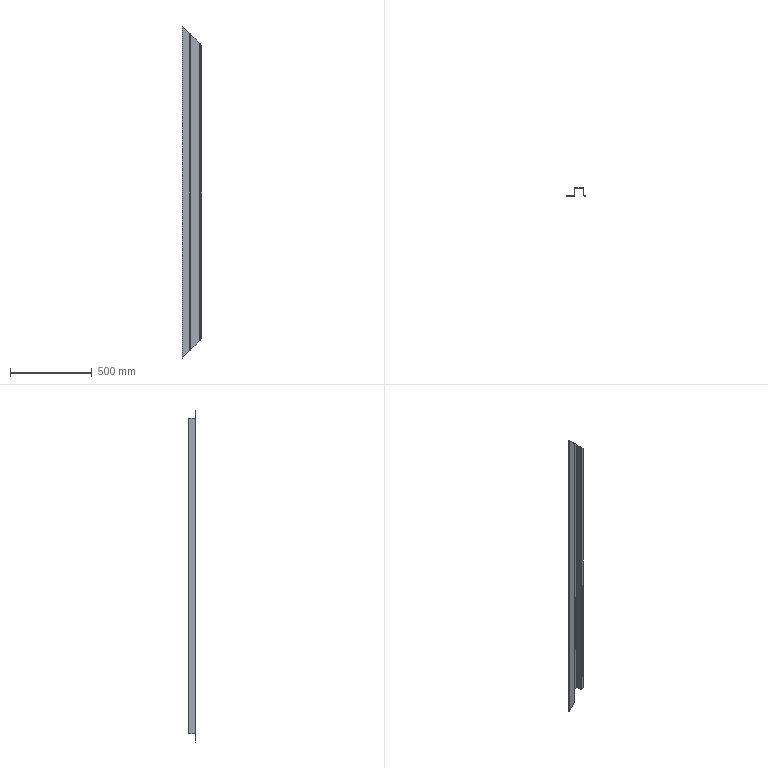Part | STEP file | 750038412 | 1 solid | 38 faces | box 120 x 46.5 x 2028 mm | volume 584981 mm3 | plane 22 | cylinder 8 | spline 8 | commonest cylinder face diameters 3 x4 6 x4
STEP:
#1=CARTESIAN_POINT('',(-14.5,45.,-908.5));
#2=VERTEX_POINT('',#1);
#3=CARTESIAN_POINT('',(-14.5,45.,908.5));
#4=VERTEX_POINT('',#3);
#5=CARTESIAN_POINT('',(-14.5,45.,1014.));
#6=DIRECTION('',(0.,0.,1.));
#7=VECTOR('',#6,1000.);
#8=LINE('',#5,#7);
#9=EDGE_CURVE('',#2,#4,#8,.T.);
#10=ORIENTED_EDGE('',*,*,#9,.F.);
#11=CARTESIAN_POINT('',(-68.5,45.,-962.5));
#12=VERTEX_POINT('',#11);
#13=CARTESIAN_POINT('',(-68.5,45.,-962.5));
#14=DIRECTION('',(0.7071,0.,0.7071));
#15=VECTOR('',#14,1000.);
#16=LINE('',#13,#15);
#17=EDGE_CURVE('',#12,#2,#16,.T.);
#18=ORIENTED_EDGE('',*,*,#17,.F.);
#19=CARTESIAN_POINT('',(-68.5,45.,962.5));
#20=VERTEX_POINT('',#19);
#21=CARTESIAN_POINT('',(-68.5,45.,1014.));
#22=DIRECTION('',(0.,0.,-1.));
#23=VECTOR('',#22,1000.);
#24=LINE('',#21,#23);
#25=EDGE_CURVE('',#20,#12,#24,.T.);
#26=ORIENTED_EDGE('',*,*,#25,.F.);
#27=CARTESIAN_POINT('',(-14.5,45.,908.5));
#28=DIRECTION('',(-0.7071,0.,0.7071));
#29=VECTOR('',#28,1000.);
#30=LINE('',#27,#29);
#31=EDGE_CURVE('',#4,#20,#30,.T.);
#32=ORIENTED_EDGE('',*,*,#31,.F.);
#33=EDGE_LOOP('',(#10,#18,#26,#32));
#34=FACE_OUTER_BOUND('',#33,.T.);
#35=CARTESIAN_POINT('',(-11.5,45.,1014.));
#36=DIRECTION('',(0.,-1.,0.));
#37=DIRECTION('',(1.,0.,0.));
#38=AXIS2_PLACEMENT_3D('',#35,#36,#37);
#39=PLANE('',#38);
#40=ADVANCED_FACE('',(#34),#39,.F.);
#41=CARTESIAN_POINT('',(-68.5,43.5,962.5));
#42=VERTEX_POINT('',#41);
#43=CARTESIAN_POINT('',(-68.5,44.25,962.5));
#44=DIRECTION('',(0.,-1.,0.));
#45=VECTOR('',#44,1000.);
#46=LINE('',#43,#45);
#47=EDGE_CURVE('',#20,#42,#46,.T.);
#48=ORIENTED_EDGE('',*,*,#47,.T.);
#49=CARTESIAN_POINT('',(-14.5,43.5,908.5));
#50=VERTEX_POINT('',#49);
#51=CARTESIAN_POINT('',(-65.75,43.5,959.75));
#52=DIRECTION('',(0.7071,0.,-0.7071));
#53=VECTOR('',#52,1000.);
#54=LINE('',#51,#53);
#55=EDGE_CURVE('',#42,#50,#54,.T.);
#56=ORIENTED_EDGE('',*,*,#55,.T.);
#57=CARTESIAN_POINT('',(-14.5,44.25,908.5));
#58=DIRECTION('',(0.,1.,0.));
#59=VECTOR('',#58,1000.);
#60=LINE('',#57,#59);
#61=EDGE_CURVE('',#50,#4,#60,.T.);
#62=ORIENTED_EDGE('',*,*,#61,.T.);
#63=ORIENTED_EDGE('',*,*,#31,.T.);
#64=EDGE_LOOP('',(#48,#56,#62,#63));
#65=FACE_OUTER_BOUND('',#64,.T.);
#66=CARTESIAN_POINT('',(-65.75,45.,959.75));
#67=DIRECTION('',(0.7071,0.,0.7071));
#68=DIRECTION('',(0.7071,0.,-0.7071));
#69=AXIS2_PLACEMENT_3D('',#66,#67,#68);
#70=PLANE('',#69);
#71=ADVANCED_FACE('',(#65),#70,.T.);
#72=CARTESIAN_POINT('',(-11.5,42.,-905.5));
#73=VERTEX_POINT('',#72);
#74=CARTESIAN_POINT('',(-11.5,42.,-905.5));
#75=CARTESIAN_POINT('',(-11.5,43.5,-905.5));
#76=CARTESIAN_POINT('',(-12.5,45.,-906.5));
#77=CARTESIAN_POINT('',(-14.5,45.,-908.5));
#78=(BOUNDED_CURVE()B_SPLINE_CURVE(3,(#74,#75,#76,#77),.UNSPECIFIED.,.F.,.T.)B_SPLINE_CURVE_WITH_KNOTS((4,4),(0.,0.005726),.UNSPECIFIED.)CURVE()GEOMETRIC_REPRESENTATION_ITEM()RATIONAL_B_SPLINE_CURVE((1.,0.6667,0.5,0.5))REPRESENTATION_ITEM(''));
#79=EDGE_CURVE('',#73,#2,#78,.T.);
#80=ORIENTED_EDGE('',*,*,#79,.T.);
#81=ORIENTED_EDGE('',*,*,#9,.T.);
#82=CARTESIAN_POINT('',(-11.5,42.,905.5));
#83=VERTEX_POINT('',#82);
#84=CARTESIAN_POINT('',(-14.5,45.,908.5));
#85=CARTESIAN_POINT('',(-12.5,45.,906.5));
#86=CARTESIAN_POINT('',(-11.5,43.5,905.5));
#87=CARTESIAN_POINT('',(-11.5,42.,905.5));
#88=(BOUNDED_CURVE()B_SPLINE_CURVE(3,(#84,#85,#86,#87),.UNSPECIFIED.,.F.,.T.)B_SPLINE_CURVE_WITH_KNOTS((4,4),(0.,0.005675),.UNSPECIFIED.)CURVE()GEOMETRIC_REPRESENTATION_ITEM()RATIONAL_B_SPLINE_CURVE((0.5,0.5,0.6667,1.))REPRESENTATION_ITEM(''));
#89=EDGE_CURVE('',#4,#83,#88,.T.);
#90=ORIENTED_EDGE('',*,*,#89,.T.);
#91=CARTESIAN_POINT('',(-11.5,42.,1014.));
#92=DIRECTION('',(0.,0.,-1.));
#93=VECTOR('',#92,1000.);
#94=LINE('',#91,#93);
#95=EDGE_CURVE('',#83,#73,#94,.T.);
#96=ORIENTED_EDGE('',*,*,#95,.T.);
#97=EDGE_LOOP('',(#80,#81,#90,#96));
#98=FACE_OUTER_BOUND('',#97,.T.);
#99=CARTESIAN_POINT('',(-14.5,42.,1014.));
#100=DIRECTION('',(0.,0.,-1.));
#101=DIRECTION('',(-1.,0.,0.));
#102=AXIS2_PLACEMENT_3D('',#99,#100,#101);
#103=CYLINDRICAL_SURFACE('',#102,3.);
#104=ADVANCED_FACE('',(#98),#103,.T.);
#105=CARTESIAN_POINT('',(-14.5,43.5,-908.5));
#106=VERTEX_POINT('',#105);
#107=CARTESIAN_POINT('',(-14.5,45.,-908.5));
#108=DIRECTION('',(0.,-1.,0.));
#109=VECTOR('',#108,1000.);
#110=LINE('',#107,#109);
#111=EDGE_CURVE('',#2,#106,#110,.T.);
#112=ORIENTED_EDGE('',*,*,#111,.T.);
#113=CARTESIAN_POINT('',(-68.5,43.5,-962.5));
#114=VERTEX_POINT('',#113);
#115=CARTESIAN_POINT('',(948.25,43.5,54.25));
#116=DIRECTION('',(-0.7071,0.,-0.7071));
#117=VECTOR('',#116,1000.);
#118=LINE('',#115,#117);
#119=EDGE_CURVE('',#106,#114,#118,.T.);
#120=ORIENTED_EDGE('',*,*,#119,.T.);
#121=CARTESIAN_POINT('',(-68.5,44.25,-962.5));
#122=DIRECTION('',(0.,1.,0.));
#123=VECTOR('',#122,1000.);
#124=LINE('',#121,#123);
#125=EDGE_CURVE('',#114,#12,#124,.T.);
#126=ORIENTED_EDGE('',*,*,#125,.T.);
#127=ORIENTED_EDGE('',*,*,#17,.T.);
#128=EDGE_LOOP('',(#112,#120,#126,#127));
#129=FACE_OUTER_BOUND('',#128,.T.);
#130=CARTESIAN_POINT('',(948.25,45.,54.25));
#131=DIRECTION('',(0.7071,0.,-0.7071));
#132=DIRECTION('',(-0.7071,0.,-0.7071));
#133=AXIS2_PLACEMENT_3D('',#130,#131,#132);
#134=PLANE('',#133);
#135=ADVANCED_FACE('',(#129),#134,.T.);
#136=CARTESIAN_POINT('',(-71.5,42.,-964.));
#137=VERTEX_POINT('',#136);
#138=CARTESIAN_POINT('',(-68.5,45.,-962.5));
#139=CARTESIAN_POINT('',(-70.5,45.,-963.5));
#140=CARTESIAN_POINT('',(-71.5,43.5,-964.));
#141=CARTESIAN_POINT('',(-71.5,42.,-964.));
#142=(BOUNDED_CURVE()B_SPLINE_CURVE(3,(#138,#139,#140,#141),.UNSPECIFIED.,.F.,.T.)B_SPLINE_CURVE_WITH_KNOTS((4,4),(0.,0.004967),.UNSPECIFIED.)CURVE()GEOMETRIC_REPRESENTATION_ITEM()RATIONAL_B_SPLINE_CURVE((0.5,0.5,0.6667,1.))REPRESENTATION_ITEM(''));
#143=EDGE_CURVE('',#12,#137,#142,.T.);
#144=ORIENTED_EDGE('',*,*,#143,.T.);
#145=CARTESIAN_POINT('',(-71.5,42.,964.));
#146=VERTEX_POINT('',#145);
#147=CARTESIAN_POINT('',(-71.5,42.,1014.));
#148=DIRECTION('',(0.,0.,1.));
#149=VECTOR('',#148,1000.);
#150=LINE('',#147,#149);
#151=EDGE_CURVE('',#137,#146,#150,.T.);
#152=ORIENTED_EDGE('',*,*,#151,.T.);
#153=CARTESIAN_POINT('',(-71.5,42.,964.));
#154=CARTESIAN_POINT('',(-71.5,43.5,964.));
#155=CARTESIAN_POINT('',(-70.5,45.,963.5));
#156=CARTESIAN_POINT('',(-68.5,45.,962.5));
#157=(BOUNDED_CURVE()B_SPLINE_CURVE(3,(#153,#154,#155,#156),.UNSPECIFIED.,.F.,.F.)B_SPLINE_CURVE_WITH_KNOTS((4,4),(0.,0.00499),.UNSPECIFIED.)CURVE()GEOMETRIC_REPRESENTATION_ITEM()RATIONAL_B_SPLINE_CURVE((1.,0.6667,0.5,0.5))REPRESENTATION_ITEM(''));
#158=EDGE_CURVE('',#146,#20,#157,.T.);
#159=ORIENTED_EDGE('',*,*,#158,.T.);
#160=ORIENTED_EDGE('',*,*,#25,.T.);
#161=EDGE_LOOP('',(#144,#152,#159,#160));
#162=FACE_OUTER_BOUND('',#161,.T.);
#163=CARTESIAN_POINT('',(-68.5,42.,1014.));
#164=DIRECTION('',(0.,0.,-1.));
#165=DIRECTION('',(-1.,0.,0.));
#166=AXIS2_PLACEMENT_3D('',#163,#164,#165);
#167=CYLINDRICAL_SURFACE('',#166,3.);
#168=ADVANCED_FACE('',(#162),#167,.T.);
#169=CARTESIAN_POINT('',(-68.5,43.5,1014.));
#170=DIRECTION('',(0.,0.,-1.));
#171=VECTOR('',#170,1000.);
#172=LINE('',#169,#171);
#173=EDGE_CURVE('',#42,#114,#172,.T.);
#174=ORIENTED_EDGE('',*,*,#173,.T.);
#175=ORIENTED_EDGE('',*,*,#119,.F.);
#176=CARTESIAN_POINT('',(-14.5,43.5,1014.));
#177=DIRECTION('',(0.,0.,1.));
#178=VECTOR('',#177,1000.);
#179=LINE('',#176,#178);
#180=EDGE_CURVE('',#106,#50,#179,.T.);
#181=ORIENTED_EDGE('',*,*,#180,.T.);
#182=ORIENTED_EDGE('',*,*,#55,.F.);
#183=EDGE_LOOP('',(#174,#175,#181,#182));
#184=FACE_OUTER_BOUND('',#183,.T.);
#185=CARTESIAN_POINT('',(-11.5,43.5,1014.));
#186=DIRECTION('',(0.,-1.,0.));
#187=DIRECTION('',(1.,0.,0.));
#188=AXIS2_PLACEMENT_3D('',#185,#186,#187);
#189=PLANE('',#188);
#190=ADVANCED_FACE('',(#184),#189,.T.);
#191=ORIENTED_EDGE('',*,*,#79,.F.);
#192=CARTESIAN_POINT('',(-13.,42.,-905.5));
#193=VERTEX_POINT('',#192);
#194=CARTESIAN_POINT('',(-11.5,42.,-905.5));
#195=DIRECTION('',(1.,0.,0.));
#196=VECTOR('',#195,1000.);
#197=LINE('',#194,#196);
#198=EDGE_CURVE('',#193,#73,#197,.T.);
#199=ORIENTED_EDGE('',*,*,#198,.F.);
#200=CARTESIAN_POINT('',(-14.5,43.5,-908.5));
#201=CARTESIAN_POINT('',(-13.5,43.5,-906.5));
#202=CARTESIAN_POINT('',(-13.,42.75,-905.5));
#203=CARTESIAN_POINT('',(-13.,42.,-905.5));
#204=(BOUNDED_CURVE()B_SPLINE_CURVE(3,(#200,#201,#202,#203),.UNSPECIFIED.,.F.,.F.)B_SPLINE_CURVE_WITH_KNOTS((4,4),(0.,0.003921),.UNSPECIFIED.)CURVE()GEOMETRIC_REPRESENTATION_ITEM()RATIONAL_B_SPLINE_CURVE((0.5,0.5,0.6667,1.))REPRESENTATION_ITEM(''));
#205=EDGE_CURVE('',#106,#193,#204,.T.);
#206=ORIENTED_EDGE('',*,*,#205,.F.);
#207=ORIENTED_EDGE('',*,*,#111,.F.);
#208=EDGE_LOOP('',(#191,#199,#206,#207));
#209=FACE_OUTER_BOUND('',#208,.T.);
#210=CARTESIAN_POINT('',(-16.,42.,-911.5));
#211=CARTESIAN_POINT('',(-16.5,42.,-911.5));
#212=CARTESIAN_POINT('',(-17.,42.,-911.5));
#213=CARTESIAN_POINT('',(-17.5,42.,-911.5));
#214=CARTESIAN_POINT('',(-16.,45.,-911.5));
#215=CARTESIAN_POINT('',(-16.5,46.,-911.5));
#216=CARTESIAN_POINT('',(-17.,47.,-911.5));
#217=CARTESIAN_POINT('',(-17.5,48.,-911.5));
#218=CARTESIAN_POINT('',(-13.,45.,-905.5));
#219=CARTESIAN_POINT('',(-12.5,46.,-905.5));
#220=CARTESIAN_POINT('',(-12.,47.,-905.5));
#221=CARTESIAN_POINT('',(-11.5,48.,-905.5));
#222=CARTESIAN_POINT('',(-13.,42.,-905.5));
#223=CARTESIAN_POINT('',(-12.5,42.,-905.5));
#224=CARTESIAN_POINT('',(-12.,42.,-905.5));
#225=CARTESIAN_POINT('',(-11.5,42.,-905.5));
#226=CARTESIAN_POINT('',(-13.,39.,-905.5));
#227=CARTESIAN_POINT('',(-12.5,38.,-905.5));
#228=CARTESIAN_POINT('',(-12.,37.,-905.5));
#229=CARTESIAN_POINT('',(-11.5,36.,-905.5));
#230=CARTESIAN_POINT('',(-16.,39.,-911.5));
#231=CARTESIAN_POINT('',(-16.5,38.,-911.5));
#232=CARTESIAN_POINT('',(-17.,37.,-911.5));
#233=CARTESIAN_POINT('',(-17.5,36.,-911.5));
#234=CARTESIAN_POINT('',(-16.,42.,-911.5));
#235=CARTESIAN_POINT('',(-16.5,42.,-911.5));
#236=CARTESIAN_POINT('',(-17.,42.,-911.5));
#237=CARTESIAN_POINT('',(-17.5,42.,-911.5));
#238=(BOUNDED_SURFACE()B_SPLINE_SURFACE(3,3,((#210,#211,#212,#213),(#214,#215,#216,#217),(#218,#219,#220,#221),(#222,#223,#224,#225),(#226,#227,#228,#229),(#230,#231,#232,#233),(#234,#235,#236,#237)),.UNSPECIFIED.,.T.,.F.,.F.)B_SPLINE_SURFACE_WITH_KNOTS((4,3,4),(4,4),(0.,0.5,1.),(0.,1.),.UNSPECIFIED.)GEOMETRIC_REPRESENTATION_ITEM()RATIONAL_B_SPLINE_SURFACE(((1.,1.,1.,1.),(0.3333,0.3333,0.3333,0.3333),(0.3333,0.3333,0.3333,0.3333),(1.,1.,1.,1.),(0.3333,0.3333,0.3333,0.3333),(0.3333,0.3333,0.3333,0.3333),(1.,1.,1.,1.)))REPRESENTATION_ITEM('')SURFACE());
#239=ADVANCED_FACE('',(#209),#238,.F.);
#240=CARTESIAN_POINT('',(-11.5,1.5,-905.5));
#241=VERTEX_POINT('',#240);
#242=CARTESIAN_POINT('',(-11.5,1.5,905.5));
#243=VERTEX_POINT('',#242);
#244=CARTESIAN_POINT('',(-11.5,1.5,1014.));
#245=DIRECTION('',(0.,0.,1.));
#246=VECTOR('',#245,1000.);
#247=LINE('',#244,#246);
#248=EDGE_CURVE('',#241,#243,#247,.T.);
#249=ORIENTED_EDGE('',*,*,#248,.F.);
#250=CARTESIAN_POINT('',(-11.5,0.,-905.5));
#251=DIRECTION('',(0.,-1.,0.));
#252=VECTOR('',#251,1000.);
#253=LINE('',#250,#252);
#254=EDGE_CURVE('',#73,#241,#253,.T.);
#255=ORIENTED_EDGE('',*,*,#254,.F.);
#256=ORIENTED_EDGE('',*,*,#95,.F.);
#257=CARTESIAN_POINT('',(-11.5,0.,905.5));
#258=DIRECTION('',(0.,1.,0.));
#259=VECTOR('',#258,1000.);
#260=LINE('',#257,#259);
#261=EDGE_CURVE('',#243,#83,#260,.T.);
#262=ORIENTED_EDGE('',*,*,#261,.F.);
#263=EDGE_LOOP('',(#249,#255,#256,#262));
#264=FACE_OUTER_BOUND('',#263,.T.);
#265=CARTESIAN_POINT('',(-11.5,0.,1014.));
#266=DIRECTION('',(-1.,0.,0.));
#267=DIRECTION('',(0.,0.,1.));
#268=AXIS2_PLACEMENT_3D('',#265,#266,#267);
#269=PLANE('',#268);
#270=ADVANCED_FACE('',(#264),#269,.F.);
#271=ORIENTED_EDGE('',*,*,#89,.F.);
#272=ORIENTED_EDGE('',*,*,#61,.F.);
#273=CARTESIAN_POINT('',(-13.,42.,905.5));
#274=VERTEX_POINT('',#273);
#275=CARTESIAN_POINT('',(-13.,42.,905.5));
#276=CARTESIAN_POINT('',(-13.,42.75,905.5));
#277=CARTESIAN_POINT('',(-13.5,43.5,906.5));
#278=CARTESIAN_POINT('',(-14.5,43.5,908.5));
#279=(BOUNDED_CURVE()B_SPLINE_CURVE(3,(#275,#276,#277,#278),.UNSPECIFIED.,.F.,.F.)B_SPLINE_CURVE_WITH_KNOTS((4,4),(0.,0.003968),.UNSPECIFIED.)CURVE()GEOMETRIC_REPRESENTATION_ITEM()RATIONAL_B_SPLINE_CURVE((1.,0.6667,0.5,0.5))REPRESENTATION_ITEM(''));
#280=EDGE_CURVE('',#274,#50,#279,.T.);
#281=ORIENTED_EDGE('',*,*,#280,.F.);
#282=CARTESIAN_POINT('',(-12.25,42.,905.5));
#283=DIRECTION('',(-1.,0.,0.));
#284=VECTOR('',#283,1000.);
#285=LINE('',#282,#284);
#286=EDGE_CURVE('',#83,#274,#285,.T.);
#287=ORIENTED_EDGE('',*,*,#286,.F.);
#288=EDGE_LOOP('',(#271,#272,#281,#287));
#289=FACE_OUTER_BOUND('',#288,.T.);
#290=CARTESIAN_POINT('',(-13.,42.,905.5));
#291=CARTESIAN_POINT('',(-12.5,42.,905.5));
#292=CARTESIAN_POINT('',(-12.,42.,905.5));
#293=CARTESIAN_POINT('',(-11.5,42.,905.5));
#294=CARTESIAN_POINT('',(-13.,45.,905.5));
#295=CARTESIAN_POINT('',(-12.5,46.,905.5));
#296=CARTESIAN_POINT('',(-12.,47.,905.5));
#297=CARTESIAN_POINT('',(-11.5,48.,905.5));
#298=CARTESIAN_POINT('',(-16.,45.,911.5));
#299=CARTESIAN_POINT('',(-16.5,46.,911.5));
#300=CARTESIAN_POINT('',(-17.,47.,911.5));
#301=CARTESIAN_POINT('',(-17.5,48.,911.5));
#302=CARTESIAN_POINT('',(-16.,42.,911.5));
#303=CARTESIAN_POINT('',(-16.5,42.,911.5));
#304=CARTESIAN_POINT('',(-17.,42.,911.5));
#305=CARTESIAN_POINT('',(-17.5,42.,911.5));
#306=CARTESIAN_POINT('',(-16.,39.,911.5));
#307=CARTESIAN_POINT('',(-16.5,38.,911.5));
#308=CARTESIAN_POINT('',(-17.,37.,911.5));
#309=CARTESIAN_POINT('',(-17.5,36.,911.5));
#310=CARTESIAN_POINT('',(-13.,39.,905.5));
#311=CARTESIAN_POINT('',(-12.5,38.,905.5));
#312=CARTESIAN_POINT('',(-12.,37.,905.5));
#313=CARTESIAN_POINT('',(-11.5,36.,905.5));
#314=CARTESIAN_POINT('',(-13.,42.,905.5));
#315=CARTESIAN_POINT('',(-12.5,42.,905.5));
#316=CARTESIAN_POINT('',(-12.,42.,905.5));
#317=CARTESIAN_POINT('',(-11.5,42.,905.5));
#318=(BOUNDED_SURFACE()B_SPLINE_SURFACE(3,3,((#290,#291,#292,#293),(#294,#295,#296,#297),(#298,#299,#300,#301),(#302,#303,#304,#305),(#306,#307,#308,#309),(#310,#311,#312,#313),(#314,#315,#316,#317)),.UNSPECIFIED.,.T.,.F.,.F.)B_SPLINE_SURFACE_WITH_KNOTS((4,3,4),(4,4),(0.,0.5,1.),(0.,1.),.UNSPECIFIED.)GEOMETRIC_REPRESENTATION_ITEM()RATIONAL_B_SPLINE_SURFACE(((1.,1.,1.,1.),(0.3333,0.3333,0.3333,0.3333),(0.3333,0.3333,0.3333,0.3333),(1.,1.,1.,1.),(0.3333,0.3333,0.3333,0.3333),(0.3333,0.3333,0.3333,0.3333),(1.,1.,1.,1.)))REPRESENTATION_ITEM('')SURFACE());
#319=ADVANCED_FACE('',(#289),#318,.F.);
#320=ORIENTED_EDGE('',*,*,#151,.F.);
#321=CARTESIAN_POINT('',(-71.5,1.5,-964.));
#322=VERTEX_POINT('',#321);
#323=CARTESIAN_POINT('',(-71.5,45.,-964.));
#324=DIRECTION('',(0.,1.,0.));
#325=VECTOR('',#324,1000.);
#326=LINE('',#323,#325);
#327=EDGE_CURVE('',#322,#137,#326,.T.);
#328=ORIENTED_EDGE('',*,*,#327,.F.);
#329=CARTESIAN_POINT('',(-71.5,1.5,964.));
#330=VERTEX_POINT('',#329);
#331=CARTESIAN_POINT('',(-71.5,1.5,1014.));
#332=DIRECTION('',(0.,0.,-1.));
#333=VECTOR('',#332,1000.);
#334=LINE('',#331,#333);
#335=EDGE_CURVE('',#330,#322,#334,.T.);
#336=ORIENTED_EDGE('',*,*,#335,.F.);
#337=CARTESIAN_POINT('',(-71.5,45.,964.));
#338=DIRECTION('',(0.,-1.,0.));
#339=VECTOR('',#338,1000.);
#340=LINE('',#337,#339);
#341=EDGE_CURVE('',#146,#330,#340,.T.);
#342=ORIENTED_EDGE('',*,*,#341,.F.);
#343=EDGE_LOOP('',(#320,#328,#336,#342));
#344=FACE_OUTER_BOUND('',#343,.T.);
#345=CARTESIAN_POINT('',(-71.5,45.,1014.));
#346=DIRECTION('',(1.,0.,0.));
#347=DIRECTION('',(0.,0.,-1.));
#348=AXIS2_PLACEMENT_3D('',#345,#346,#347);
#349=PLANE('',#348);
#350=ADVANCED_FACE('',(#344),#349,.F.);
#351=CARTESIAN_POINT('',(-70.,42.,-964.));
#352=VERTEX_POINT('',#351);
#353=CARTESIAN_POINT('',(-70.,42.,-964.));
#354=CARTESIAN_POINT('',(-70.,42.75,-964.));
#355=CARTESIAN_POINT('',(-69.5,43.5,-963.5));
#356=CARTESIAN_POINT('',(-68.5,43.5,-962.5));
#357=(BOUNDED_CURVE()B_SPLINE_CURVE(3,(#353,#354,#355,#356),.UNSPECIFIED.,.F.,.F.)B_SPLINE_CURVE_WITH_KNOTS((4,4),(0.,0.002854),.UNSPECIFIED.)CURVE()GEOMETRIC_REPRESENTATION_ITEM()RATIONAL_B_SPLINE_CURVE((1.,0.6667,0.5,0.5))REPRESENTATION_ITEM(''));
#358=EDGE_CURVE('',#352,#114,#357,.T.);
#359=ORIENTED_EDGE('',*,*,#358,.F.);
#360=CARTESIAN_POINT('',(-70.75,42.,-964.));
#361=DIRECTION('',(1.,0.,0.));
#362=VECTOR('',#361,1000.);
#363=LINE('',#360,#362);
#364=EDGE_CURVE('',#137,#352,#363,.T.);
#365=ORIENTED_EDGE('',*,*,#364,.F.);
#366=ORIENTED_EDGE('',*,*,#143,.F.);
#367=ORIENTED_EDGE('',*,*,#125,.F.);
#368=EDGE_LOOP('',(#359,#365,#366,#367));
#369=FACE_OUTER_BOUND('',#368,.T.);
#370=CARTESIAN_POINT('',(-70.,42.,-964.));
#371=CARTESIAN_POINT('',(-70.5,42.,-964.));
#372=CARTESIAN_POINT('',(-71.,42.,-964.));
#373=CARTESIAN_POINT('',(-71.5,42.,-964.));
#374=CARTESIAN_POINT('',(-70.,45.,-964.));
#375=CARTESIAN_POINT('',(-70.5,46.,-964.));
#376=CARTESIAN_POINT('',(-71.,47.,-964.));
#377=CARTESIAN_POINT('',(-71.5,48.,-964.));
#378=CARTESIAN_POINT('',(-67.,45.,-961.));
#379=CARTESIAN_POINT('',(-66.5,46.,-961.));
#380=CARTESIAN_POINT('',(-66.,47.,-961.));
#381=CARTESIAN_POINT('',(-65.5,48.,-961.));
#382=CARTESIAN_POINT('',(-67.,42.,-961.));
#383=CARTESIAN_POINT('',(-66.5,42.,-961.));
#384=CARTESIAN_POINT('',(-66.,42.,-961.));
#385=CARTESIAN_POINT('',(-65.5,42.,-961.));
#386=CARTESIAN_POINT('',(-67.,39.,-961.));
#387=CARTESIAN_POINT('',(-66.5,38.,-961.));
#388=CARTESIAN_POINT('',(-66.,37.,-961.));
#389=CARTESIAN_POINT('',(-65.5,36.,-961.));
#390=CARTESIAN_POINT('',(-70.,39.,-964.));
#391=CARTESIAN_POINT('',(-70.5,38.,-964.));
#392=CARTESIAN_POINT('',(-71.,37.,-964.));
#393=CARTESIAN_POINT('',(-71.5,36.,-964.));
#394=CARTESIAN_POINT('',(-70.,42.,-964.));
#395=CARTESIAN_POINT('',(-70.5,42.,-964.));
#396=CARTESIAN_POINT('',(-71.,42.,-964.));
#397=CARTESIAN_POINT('',(-71.5,42.,-964.));
#398=(BOUNDED_SURFACE()B_SPLINE_SURFACE(3,3,((#370,#371,#372,#373),(#374,#375,#376,#377),(#378,#379,#380,#381),(#382,#383,#384,#385),(#386,#387,#388,#389),(#390,#391,#392,#393),(#394,#395,#396,#397)),.UNSPECIFIED.,.T.,.F.,.F.)B_SPLINE_SURFACE_WITH_KNOTS((4,3,4),(4,4),(0.,0.5,1.),(0.,1.),.UNSPECIFIED.)GEOMETRIC_REPRESENTATION_ITEM()RATIONAL_B_SPLINE_SURFACE(((1.,1.,1.,1.),(0.3333,0.3333,0.3333,0.3333),(0.3333,0.3333,0.3333,0.3333),(1.,1.,1.,1.),(0.3333,0.3333,0.3333,0.3333),(0.3333,0.3333,0.3333,0.3333),(1.,1.,1.,1.)))REPRESENTATION_ITEM('')SURFACE());
#399=ADVANCED_FACE('',(#369),#398,.F.);
#400=CARTESIAN_POINT('',(-70.,42.,964.));
#401=VERTEX_POINT('',#400);
#402=CARTESIAN_POINT('',(-68.5,43.5,962.5));
#403=CARTESIAN_POINT('',(-69.5,43.5,963.5));
#404=CARTESIAN_POINT('',(-70.,42.75,964.));
#405=CARTESIAN_POINT('',(-70.,42.,964.));
#406=(BOUNDED_CURVE()B_SPLINE_CURVE(3,(#402,#403,#404,#405),.UNSPECIFIED.,.F.,.F.)B_SPLINE_CURVE_WITH_KNOTS((4,4),(0.,0.002839),.UNSPECIFIED.)CURVE()GEOMETRIC_REPRESENTATION_ITEM()RATIONAL_B_SPLINE_CURVE((0.5,0.5,0.6667,1.))REPRESENTATION_ITEM(''));
#407=EDGE_CURVE('',#42,#401,#406,.T.);
#408=ORIENTED_EDGE('',*,*,#407,.F.);
#409=ORIENTED_EDGE('',*,*,#47,.F.);
#410=ORIENTED_EDGE('',*,*,#158,.F.);
#411=CARTESIAN_POINT('',(-70.75,42.,964.));
#412=DIRECTION('',(-1.,0.,0.));
#413=VECTOR('',#412,1000.);
#414=LINE('',#411,#413);
#415=EDGE_CURVE('',#401,#146,#414,.T.);
#416=ORIENTED_EDGE('',*,*,#415,.F.);
#417=EDGE_LOOP('',(#408,#409,#410,#416));
#418=FACE_OUTER_BOUND('',#417,.T.);
#419=CARTESIAN_POINT('',(-67.,42.,961.));
#420=CARTESIAN_POINT('',(-66.5,42.,961.));
#421=CARTESIAN_POINT('',(-66.,42.,961.));
#422=CARTESIAN_POINT('',(-65.5,42.,961.));
#423=CARTESIAN_POINT('',(-67.,45.,961.));
#424=CARTESIAN_POINT('',(-66.5,46.,961.));
#425=CARTESIAN_POINT('',(-66.,47.,961.));
#426=CARTESIAN_POINT('',(-65.5,48.,961.));
#427=CARTESIAN_POINT('',(-70.,45.,964.));
#428=CARTESIAN_POINT('',(-70.5,46.,964.));
#429=CARTESIAN_POINT('',(-71.,47.,964.));
#430=CARTESIAN_POINT('',(-71.5,48.,964.));
#431=CARTESIAN_POINT('',(-70.,42.,964.));
#432=CARTESIAN_POINT('',(-70.5,42.,964.));
#433=CARTESIAN_POINT('',(-71.,42.,964.));
#434=CARTESIAN_POINT('',(-71.5,42.,964.));
#435=CARTESIAN_POINT('',(-70.,39.,964.));
#436=CARTESIAN_POINT('',(-70.5,38.,964.));
#437=CARTESIAN_POINT('',(-71.,37.,964.));
#438=CARTESIAN_POINT('',(-71.5,36.,964.));
#439=CARTESIAN_POINT('',(-67.,39.,961.));
#440=CARTESIAN_POINT('',(-66.5,38.,961.));
#441=CARTESIAN_POINT('',(-66.,37.,961.));
#442=CARTESIAN_POINT('',(-65.5,36.,961.));
#443=CARTESIAN_POINT('',(-67.,42.,961.));
#444=CARTESIAN_POINT('',(-66.5,42.,961.));
#445=CARTESIAN_POINT('',(-66.,42.,961.));
#446=CARTESIAN_POINT('',(-65.5,42.,961.));
#447=(BOUNDED_SURFACE()B_SPLINE_SURFACE(3,3,((#419,#420,#421,#422),(#423,#424,#425,#426),(#427,#428,#429,#430),(#431,#432,#433,#434),(#435,#436,#437,#438),(#439,#440,#441,#442),(#443,#444,#445,#446)),.UNSPECIFIED.,.T.,.F.,.F.)B_SPLINE_SURFACE_WITH_KNOTS((4,3,4),(4,4),(0.,0.5,1.),(0.,1.),.UNSPECIFIED.)GEOMETRIC_REPRESENTATION_ITEM()RATIONAL_B_SPLINE_SURFACE(((1.,1.,1.,1.),(0.3333,0.3333,0.3333,0.3333),(0.3333,0.3333,0.3333,0.3333),(1.,1.,1.,1.),(0.3333,0.3333,0.3333,0.3333),(0.3333,0.3333,0.3333,0.3333),(1.,1.,1.,1.)))REPRESENTATION_ITEM('')SURFACE());
#448=ADVANCED_FACE('',(#418),#447,.F.);
#449=ORIENTED_EDGE('',*,*,#407,.T.);
#450=CARTESIAN_POINT('',(-70.,42.,1014.));
#451=DIRECTION('',(0.,0.,1.));
#452=VECTOR('',#451,1000.);
#453=LINE('',#450,#452);
#454=EDGE_CURVE('',#352,#401,#453,.T.);
#455=ORIENTED_EDGE('',*,*,#454,.F.);
#456=ORIENTED_EDGE('',*,*,#358,.T.);
#457=ORIENTED_EDGE('',*,*,#173,.F.);
#458=EDGE_LOOP('',(#449,#455,#456,#457));
#459=FACE_OUTER_BOUND('',#458,.T.);
#460=CARTESIAN_POINT('',(-68.5,42.,1014.));
#461=DIRECTION('',(0.,0.,-1.));
#462=DIRECTION('',(-1.,0.,0.));
#463=AXIS2_PLACEMENT_3D('',#460,#461,#462);
#464=CYLINDRICAL_SURFACE('',#463,1.5);
#465=ADVANCED_FACE('',(#459),#464,.F.);
#466=ORIENTED_EDGE('',*,*,#280,.T.);
#467=ORIENTED_EDGE('',*,*,#180,.F.);
#468=ORIENTED_EDGE('',*,*,#205,.T.);
#469=CARTESIAN_POINT('',(-13.,42.,1014.));
#470=DIRECTION('',(0.,0.,-1.));
#471=VECTOR('',#470,1000.);
#472=LINE('',#469,#471);
#473=EDGE_CURVE('',#274,#193,#472,.T.);
#474=ORIENTED_EDGE('',*,*,#473,.F.);
#475=EDGE_LOOP('',(#466,#467,#468,#474));
#476=FACE_OUTER_BOUND('',#475,.T.);
#477=CARTESIAN_POINT('',(-14.5,42.,1014.));
#478=DIRECTION('',(0.,0.,-1.));
#479=DIRECTION('',(-1.,0.,0.));
#480=AXIS2_PLACEMENT_3D('',#477,#478,#479);
#481=CYLINDRICAL_SURFACE('',#480,1.5);
#482=ADVANCED_FACE('',(#476),#481,.F.);
#483=ORIENTED_EDGE('',*,*,#286,.T.);
#484=CARTESIAN_POINT('',(-13.,1.5,905.5));
#485=VERTEX_POINT('',#484);
#486=CARTESIAN_POINT('',(-13.,0.,905.5));
#487=DIRECTION('',(0.,-1.,0.));
#488=VECTOR('',#487,1000.);
#489=LINE('',#486,#488);
#490=EDGE_CURVE('',#274,#485,#489,.T.);
#491=ORIENTED_EDGE('',*,*,#490,.T.);
#492=CARTESIAN_POINT('',(-12.25,1.5,905.5));
#493=DIRECTION('',(1.,0.,0.));
#494=VECTOR('',#493,1000.);
#495=LINE('',#492,#494);
#496=EDGE_CURVE('',#485,#243,#495,.T.);
#497=ORIENTED_EDGE('',*,*,#496,.T.);
#498=ORIENTED_EDGE('',*,*,#261,.T.);
#499=EDGE_LOOP('',(#483,#491,#497,#498));
#500=FACE_OUTER_BOUND('',#499,.T.);
#501=CARTESIAN_POINT('',(-11.5,0.,905.5));
#502=DIRECTION('',(0.,0.,1.));
#503=DIRECTION('',(1.,0.,0.));
#504=AXIS2_PLACEMENT_3D('',#501,#502,#503);
#505=PLANE('',#504);
#506=ADVANCED_FACE('',(#500),#505,.T.);
#507=CARTESIAN_POINT('',(-10.,0.,-904.));
#508=VERTEX_POINT('',#507);
#509=CARTESIAN_POINT('',(-10.,0.,904.));
#510=VERTEX_POINT('',#509);
#511=CARTESIAN_POINT('',(-10.,0.,1014.));
#512=DIRECTION('',(0.,0.,1.));
#513=VECTOR('',#512,1000.);
#514=LINE('',#511,#513);
#515=EDGE_CURVE('',#508,#510,#514,.T.);
#516=ORIENTED_EDGE('',*,*,#515,.F.);
#517=CARTESIAN_POINT('',(-11.5,1.5,-905.5));
#518=CARTESIAN_POINT('',(-11.5,0.75,-905.5));
#519=CARTESIAN_POINT('',(-11.,0.,-905.));
#520=CARTESIAN_POINT('',(-10.,0.,-904.));
#521=(BOUNDED_CURVE()B_SPLINE_CURVE(3,(#517,#518,#519,#520),.UNSPECIFIED.,.F.,.F.)B_SPLINE_CURVE_WITH_KNOTS((4,4),(0.,0.002854),.UNSPECIFIED.)CURVE()GEOMETRIC_REPRESENTATION_ITEM()RATIONAL_B_SPLINE_CURVE((1.,0.6667,0.5,0.5))REPRESENTATION_ITEM(''));
#522=EDGE_CURVE('',#241,#508,#521,.T.);
#523=ORIENTED_EDGE('',*,*,#522,.F.);
#524=ORIENTED_EDGE('',*,*,#248,.T.);
#525=CARTESIAN_POINT('',(-10.,0.,904.));
#526=CARTESIAN_POINT('',(-11.,0.,905.));
#527=CARTESIAN_POINT('',(-11.5,0.75,905.5));
#528=CARTESIAN_POINT('',(-11.5,1.5,905.5));
#529=(BOUNDED_CURVE()B_SPLINE_CURVE(3,(#525,#526,#527,#528),.UNSPECIFIED.,.F.,.F.)B_SPLINE_CURVE_WITH_KNOTS((4,4),(0.,0.002839),.UNSPECIFIED.)CURVE()GEOMETRIC_REPRESENTATION_ITEM()RATIONAL_B_SPLINE_CURVE((0.5,0.5,0.6667,1.))REPRESENTATION_ITEM(''));
#530=EDGE_CURVE('',#510,#243,#529,.T.);
#531=ORIENTED_EDGE('',*,*,#530,.F.);
#532=EDGE_LOOP('',(#516,#523,#524,#531));
#533=FACE_OUTER_BOUND('',#532,.T.);
#534=CARTESIAN_POINT('',(-10.,1.5,1014.));
#535=DIRECTION('',(0.,0.,-1.));
#536=DIRECTION('',(-1.,0.,0.));
#537=AXIS2_PLACEMENT_3D('',#534,#535,#536);
#538=CYLINDRICAL_SURFACE('',#537,1.5);
#539=ADVANCED_FACE('',(#533),#538,.F.);
#540=CARTESIAN_POINT('',(-13.,1.5,-905.5));
#541=VERTEX_POINT('',#540);
#542=CARTESIAN_POINT('',(-11.5,1.5,-905.5));
#543=DIRECTION('',(-1.,0.,0.));
#544=VECTOR('',#543,1000.);
#545=LINE('',#542,#544);
#546=EDGE_CURVE('',#241,#541,#545,.T.);
#547=ORIENTED_EDGE('',*,*,#546,.T.);
#548=CARTESIAN_POINT('',(-13.,0.,-905.5));
#549=DIRECTION('',(0.,1.,0.));
#550=VECTOR('',#549,1000.);
#551=LINE('',#548,#550);
#552=EDGE_CURVE('',#541,#193,#551,.T.);
#553=ORIENTED_EDGE('',*,*,#552,.T.);
#554=ORIENTED_EDGE('',*,*,#198,.T.);
#555=ORIENTED_EDGE('',*,*,#254,.T.);
#556=EDGE_LOOP('',(#547,#553,#554,#555));
#557=FACE_OUTER_BOUND('',#556,.T.);
#558=CARTESIAN_POINT('',(-11.5,0.,-905.5));
#559=DIRECTION('',(0.,0.,-1.));
#560=DIRECTION('',(-1.,0.,0.));
#561=AXIS2_PLACEMENT_3D('',#558,#559,#560);
#562=PLANE('',#561);
#563=ADVANCED_FACE('',(#557),#562,.T.);
#564=ORIENTED_EDGE('',*,*,#415,.T.);
#565=ORIENTED_EDGE('',*,*,#341,.T.);
#566=CARTESIAN_POINT('',(-70.,1.5,964.));
#567=VERTEX_POINT('',#566);
#568=CARTESIAN_POINT('',(-70.75,1.5,964.));
#569=DIRECTION('',(1.,0.,0.));
#570=VECTOR('',#569,1000.);
#571=LINE('',#568,#570);
#572=EDGE_CURVE('',#330,#567,#571,.T.);
#573=ORIENTED_EDGE('',*,*,#572,.T.);
#574=CARTESIAN_POINT('',(-70.,45.,964.));
#575=DIRECTION('',(0.,1.,0.));
#576=VECTOR('',#575,1000.);
#577=LINE('',#574,#576);
#578=EDGE_CURVE('',#567,#401,#577,.T.);
#579=ORIENTED_EDGE('',*,*,#578,.T.);
#580=EDGE_LOOP('',(#564,#565,#573,#579));
#581=FACE_OUTER_BOUND('',#580,.T.);
#582=CARTESIAN_POINT('',(-70.,45.,964.));
#583=DIRECTION('',(0.,0.,1.));
#584=DIRECTION('',(1.,0.,0.));
#585=AXIS2_PLACEMENT_3D('',#582,#583,#584);
#586=PLANE('',#585);
#587=ADVANCED_FACE('',(#581),#586,.T.);
#588=CARTESIAN_POINT('',(-70.,1.5,-964.));
#589=VERTEX_POINT('',#588);
#590=CARTESIAN_POINT('',(-70.75,1.5,-964.));
#591=DIRECTION('',(-1.,0.,0.));
#592=VECTOR('',#591,1000.);
#593=LINE('',#590,#592);
#594=EDGE_CURVE('',#589,#322,#593,.T.);
#595=ORIENTED_EDGE('',*,*,#594,.T.);
#596=ORIENTED_EDGE('',*,*,#327,.T.);
#597=ORIENTED_EDGE('',*,*,#364,.T.);
#598=CARTESIAN_POINT('',(-70.,45.,-964.));
#599=DIRECTION('',(0.,-1.,0.));
#600=VECTOR('',#599,1000.);
#601=LINE('',#598,#600);
#602=EDGE_CURVE('',#352,#589,#601,.T.);
#603=ORIENTED_EDGE('',*,*,#602,.T.);
#604=EDGE_LOOP('',(#595,#596,#597,#603));
#605=FACE_OUTER_BOUND('',#604,.T.);
#606=CARTESIAN_POINT('',(-70.,45.,-964.));
#607=DIRECTION('',(0.,0.,-1.));
#608=DIRECTION('',(-1.,0.,0.));
#609=AXIS2_PLACEMENT_3D('',#606,#607,#608);
#610=PLANE('',#609);
#611=ADVANCED_FACE('',(#605),#610,.T.);
#612=ORIENTED_EDGE('',*,*,#335,.T.);
#613=CARTESIAN_POINT('',(-73.,0.,-967.));
#614=VERTEX_POINT('',#613);
#615=CARTESIAN_POINT('',(-73.,0.,-967.));
#616=CARTESIAN_POINT('',(-72.,0.,-965.));
#617=CARTESIAN_POINT('',(-71.5,0.75,-964.));
#618=CARTESIAN_POINT('',(-71.5,1.5,-964.));
#619=(BOUNDED_CURVE()B_SPLINE_CURVE(3,(#615,#616,#617,#618),.UNSPECIFIED.,.F.,.F.)B_SPLINE_CURVE_WITH_KNOTS((4,4),(0.,0.003921),.UNSPECIFIED.)CURVE()GEOMETRIC_REPRESENTATION_ITEM()RATIONAL_B_SPLINE_CURVE((0.5,0.5,0.6667,1.))REPRESENTATION_ITEM(''));
#620=EDGE_CURVE('',#614,#322,#619,.T.);
#621=ORIENTED_EDGE('',*,*,#620,.F.);
#622=CARTESIAN_POINT('',(-73.,0.,967.));
#623=VERTEX_POINT('',#622);
#624=CARTESIAN_POINT('',(-73.,0.,1014.));
#625=DIRECTION('',(0.,0.,-1.));
#626=VECTOR('',#625,1000.);
#627=LINE('',#624,#626);
#628=EDGE_CURVE('',#623,#614,#627,.T.);
#629=ORIENTED_EDGE('',*,*,#628,.F.);
#630=CARTESIAN_POINT('',(-71.5,1.5,964.));
#631=CARTESIAN_POINT('',(-71.5,0.75,964.));
#632=CARTESIAN_POINT('',(-72.,0.,965.));
#633=CARTESIAN_POINT('',(-73.,0.,967.));
#634=(BOUNDED_CURVE()B_SPLINE_CURVE(3,(#630,#631,#632,#633),.UNSPECIFIED.,.F.,.F.)B_SPLINE_CURVE_WITH_KNOTS((4,4),(0.,0.003968),.UNSPECIFIED.)CURVE()GEOMETRIC_REPRESENTATION_ITEM()RATIONAL_B_SPLINE_CURVE((1.,0.6667,0.5,0.5))REPRESENTATION_ITEM(''));
#635=EDGE_CURVE('',#330,#623,#634,.T.);
#636=ORIENTED_EDGE('',*,*,#635,.F.);
#637=EDGE_LOOP('',(#612,#621,#629,#636));
#638=FACE_OUTER_BOUND('',#637,.T.);
#639=CARTESIAN_POINT('',(-73.,1.5,1014.));
#640=DIRECTION('',(0.,0.,-1.));
#641=DIRECTION('',(-1.,0.,0.));
#642=AXIS2_PLACEMENT_3D('',#639,#640,#641);
#643=CYLINDRICAL_SURFACE('',#642,1.5);
#644=ADVANCED_FACE('',(#638),#643,.F.);
#645=CARTESIAN_POINT('',(-70.,1.5,1014.));
#646=DIRECTION('',(0.,0.,-1.));
#647=VECTOR('',#646,1000.);
#648=LINE('',#645,#647);
#649=EDGE_CURVE('',#567,#589,#648,.T.);
#650=ORIENTED_EDGE('',*,*,#649,.T.);
#651=ORIENTED_EDGE('',*,*,#602,.F.);
#652=ORIENTED_EDGE('',*,*,#454,.T.);
#653=ORIENTED_EDGE('',*,*,#578,.F.);
#654=EDGE_LOOP('',(#650,#651,#652,#653));
#655=FACE_OUTER_BOUND('',#654,.T.);
#656=CARTESIAN_POINT('',(-70.,45.,1014.));
#657=DIRECTION('',(1.,0.,0.));
#658=DIRECTION('',(0.,0.,-1.));
#659=AXIS2_PLACEMENT_3D('',#656,#657,#658);
#660=PLANE('',#659);
#661=ADVANCED_FACE('',(#655),#660,.T.);
#662=ORIENTED_EDGE('',*,*,#473,.T.);
#663=ORIENTED_EDGE('',*,*,#552,.F.);
#664=CARTESIAN_POINT('',(-13.,1.5,1014.));
#665=DIRECTION('',(0.,0.,1.));
#666=VECTOR('',#665,1000.);
#667=LINE('',#664,#666);
#668=EDGE_CURVE('',#541,#485,#667,.T.);
#669=ORIENTED_EDGE('',*,*,#668,.T.);
#670=ORIENTED_EDGE('',*,*,#490,.F.);
#671=EDGE_LOOP('',(#662,#663,#669,#670));
#672=FACE_OUTER_BOUND('',#671,.T.);
#673=CARTESIAN_POINT('',(-13.,0.,1014.));
#674=DIRECTION('',(-1.,0.,0.));
#675=DIRECTION('',(0.,0.,1.));
#676=AXIS2_PLACEMENT_3D('',#673,#674,#675);
#677=PLANE('',#676);
#678=ADVANCED_FACE('',(#672),#677,.T.);
#679=ORIENTED_EDGE('',*,*,#530,.T.);
#680=ORIENTED_EDGE('',*,*,#496,.F.);
#681=CARTESIAN_POINT('',(-10.,-1.5,904.));
#682=VERTEX_POINT('',#681);
#683=CARTESIAN_POINT('',(-10.,-1.5,904.));
#684=CARTESIAN_POINT('',(-12.,-1.5,905.));
#685=CARTESIAN_POINT('',(-13.,0.,905.5));
#686=CARTESIAN_POINT('',(-13.,1.5,905.5));
#687=(BOUNDED_CURVE()B_SPLINE_CURVE(3,(#683,#684,#685,#686),.UNSPECIFIED.,.F.,.F.)B_SPLINE_CURVE_WITH_KNOTS((4,4),(0.,0.004981),.UNSPECIFIED.)CURVE()GEOMETRIC_REPRESENTATION_ITEM()RATIONAL_B_SPLINE_CURVE((0.5,0.5,0.6667,1.))REPRESENTATION_ITEM(''));
#688=EDGE_CURVE('',#682,#485,#687,.T.);
#689=ORIENTED_EDGE('',*,*,#688,.F.);
#690=CARTESIAN_POINT('',(-10.,0.,904.));
#691=DIRECTION('',(0.,-1.,0.));
#692=VECTOR('',#691,1000.);
#693=LINE('',#690,#692);
#694=EDGE_CURVE('',#510,#682,#693,.T.);
#695=ORIENTED_EDGE('',*,*,#694,.F.);
#696=EDGE_LOOP('',(#679,#680,#689,#695));
#697=FACE_OUTER_BOUND('',#696,.T.);
#698=CARTESIAN_POINT('',(-7.,1.5,902.5));
#699=CARTESIAN_POINT('',(-7.5,1.5,902.5));
#700=CARTESIAN_POINT('',(-8.,1.5,902.5));
#701=CARTESIAN_POINT('',(-8.5,1.5,902.5));
#702=CARTESIAN_POINT('',(-7.,-4.5,902.5));
#703=CARTESIAN_POINT('',(-7.5,-3.5,902.5));
#704=CARTESIAN_POINT('',(-8.,-2.5,902.5));
#705=CARTESIAN_POINT('',(-8.5,-1.5,902.5));
#706=CARTESIAN_POINT('',(-13.,-4.5,905.5));
#707=CARTESIAN_POINT('',(-12.5,-3.5,905.5));
#708=CARTESIAN_POINT('',(-12.,-2.5,905.5));
#709=CARTESIAN_POINT('',(-11.5,-1.5,905.5));
#710=CARTESIAN_POINT('',(-13.,1.5,905.5));
#711=CARTESIAN_POINT('',(-12.5,1.5,905.5));
#712=CARTESIAN_POINT('',(-12.,1.5,905.5));
#713=CARTESIAN_POINT('',(-11.5,1.5,905.5));
#714=CARTESIAN_POINT('',(-13.,7.5,905.5));
#715=CARTESIAN_POINT('',(-12.5,6.5,905.5));
#716=CARTESIAN_POINT('',(-12.,5.5,905.5));
#717=CARTESIAN_POINT('',(-11.5,4.5,905.5));
#718=CARTESIAN_POINT('',(-7.,7.5,902.5));
#719=CARTESIAN_POINT('',(-7.5,6.5,902.5));
#720=CARTESIAN_POINT('',(-8.,5.5,902.5));
#721=CARTESIAN_POINT('',(-8.5,4.5,902.5));
#722=CARTESIAN_POINT('',(-7.,1.5,902.5));
#723=CARTESIAN_POINT('',(-7.5,1.5,902.5));
#724=CARTESIAN_POINT('',(-8.,1.5,902.5));
#725=CARTESIAN_POINT('',(-8.5,1.5,902.5));
#726=(BOUNDED_SURFACE()B_SPLINE_SURFACE(3,3,((#698,#699,#700,#701),(#702,#703,#704,#705),(#706,#707,#708,#709),(#710,#711,#712,#713),(#714,#715,#716,#717),(#718,#719,#720,#721),(#722,#723,#724,#725)),.UNSPECIFIED.,.T.,.F.,.T.)B_SPLINE_SURFACE_WITH_KNOTS((4,3,4),(4,4),(0.,0.5,1.),(0.,1.),.UNSPECIFIED.)GEOMETRIC_REPRESENTATION_ITEM()RATIONAL_B_SPLINE_SURFACE(((1.,1.,1.,1.),(0.3333,0.3333,0.3333,0.3333),(0.3333,0.3333,0.3333,0.3333),(1.,1.,1.,1.),(0.3333,0.3333,0.3333,0.3333),(0.3333,0.3333,0.3333,0.3333),(1.,1.,1.,1.)))REPRESENTATION_ITEM('')SURFACE());
#727=ADVANCED_FACE('',(#697),#726,.F.);
#728=CARTESIAN_POINT('',(0.,0.,-894.));
#729=VERTEX_POINT('',#728);
#730=CARTESIAN_POINT('',(0.,0.,894.));
#731=VERTEX_POINT('',#730);
#732=CARTESIAN_POINT('',(0.,0.,1014.));
#733=DIRECTION('',(0.,0.,1.));
#734=VECTOR('',#733,1000.);
#735=LINE('',#732,#734);
#736=EDGE_CURVE('',#729,#731,#735,.T.);
#737=ORIENTED_EDGE('',*,*,#736,.F.);
#738=CARTESIAN_POINT('',(-10.,0.,-904.));
#739=DIRECTION('',(0.7071,0.,0.7071));
#740=VECTOR('',#739,1000.);
#741=LINE('',#738,#740);
#742=EDGE_CURVE('',#508,#729,#741,.T.);
#743=ORIENTED_EDGE('',*,*,#742,.F.);
#744=ORIENTED_EDGE('',*,*,#515,.T.);
#745=CARTESIAN_POINT('',(0.,0.,894.));
#746=DIRECTION('',(-0.7071,0.,0.7071));
#747=VECTOR('',#746,1000.);
#748=LINE('',#745,#747);
#749=EDGE_CURVE('',#731,#510,#748,.T.);
#750=ORIENTED_EDGE('',*,*,#749,.F.);
#751=EDGE_LOOP('',(#737,#743,#744,#750));
#752=FACE_OUTER_BOUND('',#751,.T.);
#753=CARTESIAN_POINT('',(0.,0.,1014.));
#754=DIRECTION('',(0.,-1.,0.));
#755=DIRECTION('',(0.,0.,-1.));
#756=AXIS2_PLACEMENT_3D('',#753,#754,#755);
#757=PLANE('',#756);
#758=ADVANCED_FACE('',(#752),#757,.F.);
#759=ORIENTED_EDGE('',*,*,#522,.T.);
#760=CARTESIAN_POINT('',(-10.,-1.5,-904.));
#761=VERTEX_POINT('',#760);
#762=CARTESIAN_POINT('',(-10.,-0.75,-904.));
#763=DIRECTION('',(0.,1.,0.));
#764=VECTOR('',#763,1000.);
#765=LINE('',#762,#764);
#766=EDGE_CURVE('',#761,#508,#765,.T.);
#767=ORIENTED_EDGE('',*,*,#766,.F.);
#768=CARTESIAN_POINT('',(-13.,1.5,-905.5));
#769=CARTESIAN_POINT('',(-13.,0.,-905.5));
#770=CARTESIAN_POINT('',(-12.,-1.5,-905.));
#771=CARTESIAN_POINT('',(-10.,-1.5,-904.));
#772=(BOUNDED_CURVE()B_SPLINE_CURVE(3,(#768,#769,#770,#771),.UNSPECIFIED.,.F.,.F.)B_SPLINE_CURVE_WITH_KNOTS((4,4),(0.,0.00497),.UNSPECIFIED.)CURVE()GEOMETRIC_REPRESENTATION_ITEM()RATIONAL_B_SPLINE_CURVE((1.,0.6667,0.5,0.5))REPRESENTATION_ITEM(''));
#773=EDGE_CURVE('',#541,#761,#772,.T.);
#774=ORIENTED_EDGE('',*,*,#773,.F.);
#775=ORIENTED_EDGE('',*,*,#546,.F.);
#776=EDGE_LOOP('',(#759,#767,#774,#775));
#777=FACE_OUTER_BOUND('',#776,.T.);
#778=CARTESIAN_POINT('',(-13.,1.5,-905.5));
#779=CARTESIAN_POINT('',(-12.5,1.5,-905.5));
#780=CARTESIAN_POINT('',(-12.,1.5,-905.5));
#781=CARTESIAN_POINT('',(-11.5,1.5,-905.5));
#782=CARTESIAN_POINT('',(-13.,-4.5,-905.5));
#783=CARTESIAN_POINT('',(-12.5,-3.5,-905.5));
#784=CARTESIAN_POINT('',(-12.,-2.5,-905.5));
#785=CARTESIAN_POINT('',(-11.5,-1.5,-905.5));
#786=CARTESIAN_POINT('',(-7.,-4.5,-902.5));
#787=CARTESIAN_POINT('',(-7.5,-3.5,-902.5));
#788=CARTESIAN_POINT('',(-8.,-2.5,-902.5));
#789=CARTESIAN_POINT('',(-8.5,-1.5,-902.5));
#790=CARTESIAN_POINT('',(-7.,1.5,-902.5));
#791=CARTESIAN_POINT('',(-7.5,1.5,-902.5));
#792=CARTESIAN_POINT('',(-8.,1.5,-902.5));
#793=CARTESIAN_POINT('',(-8.5,1.5,-902.5));
#794=CARTESIAN_POINT('',(-7.,7.5,-902.5));
#795=CARTESIAN_POINT('',(-7.5,6.5,-902.5));
#796=CARTESIAN_POINT('',(-8.,5.5,-902.5));
#797=CARTESIAN_POINT('',(-8.5,4.5,-902.5));
#798=CARTESIAN_POINT('',(-13.,7.5,-905.5));
#799=CARTESIAN_POINT('',(-12.5,6.5,-905.5));
#800=CARTESIAN_POINT('',(-12.,5.5,-905.5));
#801=CARTESIAN_POINT('',(-11.5,4.5,-905.5));
#802=CARTESIAN_POINT('',(-13.,1.5,-905.5));
#803=CARTESIAN_POINT('',(-12.5,1.5,-905.5));
#804=CARTESIAN_POINT('',(-12.,1.5,-905.5));
#805=CARTESIAN_POINT('',(-11.5,1.5,-905.5));
#806=(BOUNDED_SURFACE()B_SPLINE_SURFACE(3,3,((#778,#779,#780,#781),(#782,#783,#784,#785),(#786,#787,#788,#789),(#790,#791,#792,#793),(#794,#795,#796,#797),(#798,#799,#800,#801),(#802,#803,#804,#805)),.UNSPECIFIED.,.T.,.F.,.F.)B_SPLINE_SURFACE_WITH_KNOTS((4,3,4),(4,4),(0.,0.5,1.),(0.,1.),.UNSPECIFIED.)GEOMETRIC_REPRESENTATION_ITEM()RATIONAL_B_SPLINE_SURFACE(((1.,1.,1.,1.),(0.3333,0.3333,0.3333,0.3333),(0.3333,0.3333,0.3333,0.3333),(1.,1.,1.,1.),(0.3333,0.3333,0.3333,0.3333),(0.3333,0.3333,0.3333,0.3333),(1.,1.,1.,1.)))REPRESENTATION_ITEM('')SURFACE());
#807=ADVANCED_FACE('',(#777),#806,.F.);
#808=CARTESIAN_POINT('',(-73.,-1.5,967.));
#809=VERTEX_POINT('',#808);
#810=CARTESIAN_POINT('',(-73.,0.,967.));
#811=DIRECTION('',(0.,1.,0.));
#812=VECTOR('',#811,1000.);
#813=LINE('',#810,#812);
#814=EDGE_CURVE('',#809,#623,#813,.T.);
#815=ORIENTED_EDGE('',*,*,#814,.F.);
#816=CARTESIAN_POINT('',(-70.,1.5,964.));
#817=CARTESIAN_POINT('',(-70.,0.,964.));
#818=CARTESIAN_POINT('',(-71.,-1.5,965.));
#819=CARTESIAN_POINT('',(-73.,-1.5,967.));
#820=(BOUNDED_CURVE()B_SPLINE_CURVE(3,(#816,#817,#818,#819),.UNSPECIFIED.,.F.,.F.)B_SPLINE_CURVE_WITH_KNOTS((4,4),(0.,0.005725),.UNSPECIFIED.)CURVE()GEOMETRIC_REPRESENTATION_ITEM()RATIONAL_B_SPLINE_CURVE((1.,0.6667,0.5,0.5))REPRESENTATION_ITEM(''));
#821=EDGE_CURVE('',#567,#809,#820,.T.);
#822=ORIENTED_EDGE('',*,*,#821,.F.);
#823=ORIENTED_EDGE('',*,*,#572,.F.);
#824=ORIENTED_EDGE('',*,*,#635,.T.);
#825=EDGE_LOOP('',(#815,#822,#823,#824));
#826=FACE_OUTER_BOUND('',#825,.T.);
#827=CARTESIAN_POINT('',(-70.,1.5,964.));
#828=CARTESIAN_POINT('',(-70.5,1.5,964.));
#829=CARTESIAN_POINT('',(-71.,1.5,964.));
#830=CARTESIAN_POINT('',(-71.5,1.5,964.));
#831=CARTESIAN_POINT('',(-70.,-4.5,964.));
#832=CARTESIAN_POINT('',(-70.5,-3.5,964.));
#833=CARTESIAN_POINT('',(-71.,-2.5,964.));
#834=CARTESIAN_POINT('',(-71.5,-1.5,964.));
#835=CARTESIAN_POINT('',(-76.,-4.5,970.));
#836=CARTESIAN_POINT('',(-75.5,-3.5,970.));
#837=CARTESIAN_POINT('',(-75.,-2.5,970.));
#838=CARTESIAN_POINT('',(-74.5,-1.5,970.));
#839=CARTESIAN_POINT('',(-76.,1.5,970.));
#840=CARTESIAN_POINT('',(-75.5,1.5,970.));
#841=CARTESIAN_POINT('',(-75.,1.5,970.));
#842=CARTESIAN_POINT('',(-74.5,1.5,970.));
#843=CARTESIAN_POINT('',(-76.,7.5,970.));
#844=CARTESIAN_POINT('',(-75.5,6.5,970.));
#845=CARTESIAN_POINT('',(-75.,5.5,970.));
#846=CARTESIAN_POINT('',(-74.5,4.5,970.));
#847=CARTESIAN_POINT('',(-70.,7.5,964.));
#848=CARTESIAN_POINT('',(-70.5,6.5,964.));
#849=CARTESIAN_POINT('',(-71.,5.5,964.));
#850=CARTESIAN_POINT('',(-71.5,4.5,964.));
#851=CARTESIAN_POINT('',(-70.,1.5,964.));
#852=CARTESIAN_POINT('',(-70.5,1.5,964.));
#853=CARTESIAN_POINT('',(-71.,1.5,964.));
#854=CARTESIAN_POINT('',(-71.5,1.5,964.));
#855=(BOUNDED_SURFACE()B_SPLINE_SURFACE(3,3,((#827,#828,#829,#830),(#831,#832,#833,#834),(#835,#836,#837,#838),(#839,#840,#841,#842),(#843,#844,#845,#846),(#847,#848,#849,#850),(#851,#852,#853,#854)),.UNSPECIFIED.,.T.,.F.,.F.)B_SPLINE_SURFACE_WITH_KNOTS((4,3,4),(4,4),(0.,0.5,1.),(0.,1.),.UNSPECIFIED.)GEOMETRIC_REPRESENTATION_ITEM()RATIONAL_B_SPLINE_SURFACE(((1.,1.,1.,1.),(0.3333,0.3333,0.3333,0.3333),(0.3333,0.3333,0.3333,0.3333),(1.,1.,1.,1.),(0.3333,0.3333,0.3333,0.3333),(0.3333,0.3333,0.3333,0.3333),(1.,1.,1.,1.)))REPRESENTATION_ITEM('')SURFACE());
#856=ADVANCED_FACE('',(#826),#855,.F.);
#857=CARTESIAN_POINT('',(-73.,-1.5,-967.));
#858=VERTEX_POINT('',#857);
#859=CARTESIAN_POINT('',(-73.,-1.5,-967.));
#860=CARTESIAN_POINT('',(-71.,-1.5,-965.));
#861=CARTESIAN_POINT('',(-70.,0.,-964.));
#862=CARTESIAN_POINT('',(-70.,1.5,-964.));
#863=(BOUNDED_CURVE()B_SPLINE_CURVE(3,(#859,#860,#861,#862),.UNSPECIFIED.,.F.,.T.)B_SPLINE_CURVE_WITH_KNOTS((4,4),(0.,0.005675),.UNSPECIFIED.)CURVE()GEOMETRIC_REPRESENTATION_ITEM()RATIONAL_B_SPLINE_CURVE((0.5,0.5,0.6667,1.))REPRESENTATION_ITEM(''));
#864=EDGE_CURVE('',#858,#589,#863,.T.);
#865=ORIENTED_EDGE('',*,*,#864,.F.);
#866=CARTESIAN_POINT('',(-73.,0.,-967.));
#867=DIRECTION('',(0.,-1.,0.));
#868=VECTOR('',#867,1000.);
#869=LINE('',#866,#868);
#870=EDGE_CURVE('',#614,#858,#869,.T.);
#871=ORIENTED_EDGE('',*,*,#870,.F.);
#872=ORIENTED_EDGE('',*,*,#620,.T.);
#873=ORIENTED_EDGE('',*,*,#594,.F.);
#874=EDGE_LOOP('',(#865,#871,#872,#873));
#875=FACE_OUTER_BOUND('',#874,.T.);
#876=CARTESIAN_POINT('',(-76.,1.5,-970.));
#877=CARTESIAN_POINT('',(-75.5,1.5,-970.));
#878=CARTESIAN_POINT('',(-75.,1.5,-970.));
#879=CARTESIAN_POINT('',(-74.5,1.5,-970.));
#880=CARTESIAN_POINT('',(-76.,-4.5,-970.));
#881=CARTESIAN_POINT('',(-75.5,-3.5,-970.));
#882=CARTESIAN_POINT('',(-75.,-2.5,-970.));
#883=CARTESIAN_POINT('',(-74.5,-1.5,-970.));
#884=CARTESIAN_POINT('',(-70.,-4.5,-964.));
#885=CARTESIAN_POINT('',(-70.5,-3.5,-964.));
#886=CARTESIAN_POINT('',(-71.,-2.5,-964.));
#887=CARTESIAN_POINT('',(-71.5,-1.5,-964.));
#888=CARTESIAN_POINT('',(-70.,1.5,-964.));
#889=CARTESIAN_POINT('',(-70.5,1.5,-964.));
#890=CARTESIAN_POINT('',(-71.,1.5,-964.));
#891=CARTESIAN_POINT('',(-71.5,1.5,-964.));
#892=CARTESIAN_POINT('',(-70.,7.5,-964.));
#893=CARTESIAN_POINT('',(-70.5,6.5,-964.));
#894=CARTESIAN_POINT('',(-71.,5.5,-964.));
#895=CARTESIAN_POINT('',(-71.5,4.5,-964.));
#896=CARTESIAN_POINT('',(-76.,7.5,-970.));
#897=CARTESIAN_POINT('',(-75.5,6.5,-970.));
#898=CARTESIAN_POINT('',(-75.,5.5,-970.));
#899=CARTESIAN_POINT('',(-74.5,4.5,-970.));
#900=CARTESIAN_POINT('',(-76.,1.5,-970.));
#901=CARTESIAN_POINT('',(-75.5,1.5,-970.));
#902=CARTESIAN_POINT('',(-75.,1.5,-970.));
#903=CARTESIAN_POINT('',(-74.5,1.5,-970.));
#904=(BOUNDED_SURFACE()B_SPLINE_SURFACE(3,3,((#876,#877,#878,#879),(#880,#881,#882,#883),(#884,#885,#886,#887),(#888,#889,#890,#891),(#892,#893,#894,#895),(#896,#897,#898,#899),(#900,#901,#902,#903)),.UNSPECIFIED.,.T.,.F.,.F.)B_SPLINE_SURFACE_WITH_KNOTS((4,3,4),(4,4),(0.,0.5,1.),(0.,1.),.UNSPECIFIED.)GEOMETRIC_REPRESENTATION_ITEM()RATIONAL_B_SPLINE_SURFACE(((1.,1.,1.,1.),(0.3333,0.3333,0.3333,0.3333),(0.3333,0.3333,0.3333,0.3333),(1.,1.,1.,1.),(0.3333,0.3333,0.3333,0.3333),(0.3333,0.3333,0.3333,0.3333),(1.,1.,1.,1.)))REPRESENTATION_ITEM('')SURFACE());
#905=ADVANCED_FACE('',(#875),#904,.F.);
#906=ORIENTED_EDGE('',*,*,#628,.T.);
#907=CARTESIAN_POINT('',(-120.,0.,-1014.));
#908=VERTEX_POINT('',#907);
#909=CARTESIAN_POINT('',(-120.,0.,-1014.));
#910=DIRECTION('',(0.7071,0.,0.7071));
#911=VECTOR('',#910,1000.);
#912=LINE('',#909,#911);
#913=EDGE_CURVE('',#908,#614,#912,.T.);
#914=ORIENTED_EDGE('',*,*,#913,.F.);
#915=CARTESIAN_POINT('',(-120.,0.,1014.));
#916=VERTEX_POINT('',#915);
#917=CARTESIAN_POINT('',(-120.,0.,1014.));
#918=DIRECTION('',(0.,0.,-1.));
#919=VECTOR('',#918,1000.);
#920=LINE('',#917,#919);
#921=EDGE_CURVE('',#916,#908,#920,.T.);
#922=ORIENTED_EDGE('',*,*,#921,.F.);
#923=CARTESIAN_POINT('',(-73.,0.,967.));
#924=DIRECTION('',(-0.7071,0.,0.7071));
#925=VECTOR('',#924,1000.);
#926=LINE('',#923,#925);
#927=EDGE_CURVE('',#623,#916,#926,.T.);
#928=ORIENTED_EDGE('',*,*,#927,.F.);
#929=EDGE_LOOP('',(#906,#914,#922,#928));
#930=FACE_OUTER_BOUND('',#929,.T.);
#931=CARTESIAN_POINT('',(-71.5,0.,1014.));
#932=DIRECTION('',(0.,-1.,0.));
#933=DIRECTION('',(1.,0.,0.));
#934=AXIS2_PLACEMENT_3D('',#931,#932,#933);
#935=PLANE('',#934);
#936=ADVANCED_FACE('',(#930),#935,.F.);
#937=CARTESIAN_POINT('',(-73.,-1.5,1014.));
#938=DIRECTION('',(0.,0.,-1.));
#939=VECTOR('',#938,1000.);
#940=LINE('',#937,#939);
#941=EDGE_CURVE('',#809,#858,#940,.T.);
#942=ORIENTED_EDGE('',*,*,#941,.T.);
#943=ORIENTED_EDGE('',*,*,#864,.T.);
#944=ORIENTED_EDGE('',*,*,#649,.F.);
#945=ORIENTED_EDGE('',*,*,#821,.T.);
#946=EDGE_LOOP('',(#942,#943,#944,#945));
#947=FACE_OUTER_BOUND('',#946,.T.);
#948=CARTESIAN_POINT('',(-73.,1.5,1014.));
#949=DIRECTION('',(0.,0.,-1.));
#950=DIRECTION('',(-1.,0.,0.));
#951=AXIS2_PLACEMENT_3D('',#948,#949,#950);
#952=CYLINDRICAL_SURFACE('',#951,3.);
#953=ADVANCED_FACE('',(#947),#952,.T.);
#954=ORIENTED_EDGE('',*,*,#668,.F.);
#955=ORIENTED_EDGE('',*,*,#773,.T.);
#956=CARTESIAN_POINT('',(-10.,-1.5,1014.));
#957=DIRECTION('',(0.,0.,1.));
#958=VECTOR('',#957,1000.);
#959=LINE('',#956,#958);
#960=EDGE_CURVE('',#761,#682,#959,.T.);
#961=ORIENTED_EDGE('',*,*,#960,.T.);
#962=ORIENTED_EDGE('',*,*,#688,.T.);
#963=EDGE_LOOP('',(#954,#955,#961,#962));
#964=FACE_OUTER_BOUND('',#963,.T.);
#965=CARTESIAN_POINT('',(-10.,1.5,1014.));
#966=DIRECTION('',(0.,0.,-1.));
#967=DIRECTION('',(-1.,0.,0.));
#968=AXIS2_PLACEMENT_3D('',#965,#966,#967);
#969=CYLINDRICAL_SURFACE('',#968,3.);
#970=ADVANCED_FACE('',(#964),#969,.T.);
#971=ORIENTED_EDGE('',*,*,#694,.T.);
#972=CARTESIAN_POINT('',(0.,-1.5,894.));
#973=VERTEX_POINT('',#972);
#974=CARTESIAN_POINT('',(-60.,-1.5,954.));
#975=DIRECTION('',(0.7071,0.,-0.7071));
#976=VECTOR('',#975,1000.);
#977=LINE('',#974,#976);
#978=EDGE_CURVE('',#682,#973,#977,.T.);
#979=ORIENTED_EDGE('',*,*,#978,.T.);
#980=CARTESIAN_POINT('',(0.,0.,894.));
#981=DIRECTION('',(0.,1.,0.));
#982=VECTOR('',#981,1000.);
#983=LINE('',#980,#982);
#984=EDGE_CURVE('',#973,#731,#983,.T.);
#985=ORIENTED_EDGE('',*,*,#984,.T.);
#986=ORIENTED_EDGE('',*,*,#749,.T.);
#987=EDGE_LOOP('',(#971,#979,#985,#986));
#988=FACE_OUTER_BOUND('',#987,.T.);
#989=CARTESIAN_POINT('',(-60.,0.,954.));
#990=DIRECTION('',(0.7071,0.,0.7071));
#991=DIRECTION('',(0.7071,0.,-0.7071));
#992=AXIS2_PLACEMENT_3D('',#989,#990,#991);
#993=PLANE('',#992);
#994=ADVANCED_FACE('',(#988),#993,.T.);
#995=CARTESIAN_POINT('',(0.,-1.5,-894.));
#996=VERTEX_POINT('',#995);
#997=CARTESIAN_POINT('',(0.,-1.5,1014.));
#998=DIRECTION('',(0.,0.,1.));
#999=VECTOR('',#998,1000.);
#1000=LINE('',#997,#999);
#1001=EDGE_CURVE('',#996,#973,#1000,.T.);
#1002=ORIENTED_EDGE('',*,*,#1001,.F.);
#1003=CARTESIAN_POINT('',(0.,0.,-894.));
#1004=DIRECTION('',(0.,-1.,0.));
#1005=VECTOR('',#1004,1000.);
#1006=LINE('',#1003,#1005);
#1007=EDGE_CURVE('',#729,#996,#1006,.T.);
#1008=ORIENTED_EDGE('',*,*,#1007,.F.);
#1009=ORIENTED_EDGE('',*,*,#736,.T.);
#1010=ORIENTED_EDGE('',*,*,#984,.F.);
#1011=EDGE_LOOP('',(#1002,#1008,#1009,#1010));
#1012=FACE_OUTER_BOUND('',#1011,.T.);
#1013=CARTESIAN_POINT('',(0.,0.,1014.));
#1014=DIRECTION('',(-1.,0.,0.));
#1015=DIRECTION('',(0.,0.,1.));
#1016=AXIS2_PLACEMENT_3D('',#1013,#1014,#1015);
#1017=PLANE('',#1016);
#1018=ADVANCED_FACE('',(#1012),#1017,.F.);
#1019=ORIENTED_EDGE('',*,*,#742,.T.);
#1020=ORIENTED_EDGE('',*,*,#1007,.T.);
#1021=CARTESIAN_POINT('',(954.,-1.5,60.));
#1022=DIRECTION('',(-0.7071,0.,-0.7071));
#1023=VECTOR('',#1022,1000.);
#1024=LINE('',#1021,#1023);
#1025=EDGE_CURVE('',#996,#761,#1024,.T.);
#1026=ORIENTED_EDGE('',*,*,#1025,.T.);
#1027=ORIENTED_EDGE('',*,*,#766,.T.);
#1028=EDGE_LOOP('',(#1019,#1020,#1026,#1027));
#1029=FACE_OUTER_BOUND('',#1028,.T.);
#1030=CARTESIAN_POINT('',(954.,0.,60.));
#1031=DIRECTION('',(0.7071,0.,-0.7071));
#1032=DIRECTION('',(-0.7071,0.,-0.7071));
#1033=AXIS2_PLACEMENT_3D('',#1030,#1031,#1032);
#1034=PLANE('',#1033);
#1035=ADVANCED_FACE('',(#1029),#1034,.T.);
#1036=CARTESIAN_POINT('',(-120.,-1.5,1014.));
#1037=VERTEX_POINT('',#1036);
#1038=CARTESIAN_POINT('',(-120.,0.,1014.));
#1039=DIRECTION('',(0.,-1.,0.));
#1040=VECTOR('',#1039,1000.);
#1041=LINE('',#1038,#1040);
#1042=EDGE_CURVE('',#916,#1037,#1041,.T.);
#1043=ORIENTED_EDGE('',*,*,#1042,.T.);
#1044=CARTESIAN_POINT('',(-95.75,-1.5,989.75));
#1045=DIRECTION('',(0.7071,0.,-0.7071));
#1046=VECTOR('',#1045,1000.);
#1047=LINE('',#1044,#1046);
#1048=EDGE_CURVE('',#1037,#809,#1047,.T.);
#1049=ORIENTED_EDGE('',*,*,#1048,.T.);
#1050=ORIENTED_EDGE('',*,*,#814,.T.);
#1051=ORIENTED_EDGE('',*,*,#927,.T.);
#1052=EDGE_LOOP('',(#1043,#1049,#1050,#1051));
#1053=FACE_OUTER_BOUND('',#1052,.T.);
#1054=CARTESIAN_POINT('',(-95.75,0.,989.75));
#1055=DIRECTION('',(0.7071,0.,0.7071));
#1056=DIRECTION('',(0.7071,0.,-0.7071));
#1057=AXIS2_PLACEMENT_3D('',#1054,#1055,#1056);
#1058=PLANE('',#1057);
#1059=ADVANCED_FACE('',(#1053),#1058,.T.);
#1060=ORIENTED_EDGE('',*,*,#870,.T.);
#1061=CARTESIAN_POINT('',(-120.,-1.5,-1014.));
#1062=VERTEX_POINT('',#1061);
#1063=CARTESIAN_POINT('',(918.25,-1.5,24.25));
#1064=DIRECTION('',(-0.7071,0.,-0.7071));
#1065=VECTOR('',#1064,1000.);
#1066=LINE('',#1063,#1065);
#1067=EDGE_CURVE('',#858,#1062,#1066,.T.);
#1068=ORIENTED_EDGE('',*,*,#1067,.T.);
#1069=CARTESIAN_POINT('',(-120.,0.,-1014.));
#1070=DIRECTION('',(0.,1.,0.));
#1071=VECTOR('',#1070,1000.);
#1072=LINE('',#1069,#1071);
#1073=EDGE_CURVE('',#1062,#908,#1072,.T.);
#1074=ORIENTED_EDGE('',*,*,#1073,.T.);
#1075=ORIENTED_EDGE('',*,*,#913,.T.);
#1076=EDGE_LOOP('',(#1060,#1068,#1074,#1075));
#1077=FACE_OUTER_BOUND('',#1076,.T.);
#1078=CARTESIAN_POINT('',(918.25,0.,24.25));
#1079=DIRECTION('',(0.7071,0.,-0.7071));
#1080=DIRECTION('',(-0.7071,0.,-0.7071));
#1081=AXIS2_PLACEMENT_3D('',#1078,#1079,#1080);
#1082=PLANE('',#1081);
#1083=ADVANCED_FACE('',(#1077),#1082,.T.);
#1084=ORIENTED_EDGE('',*,*,#1073,.F.);
#1085=CARTESIAN_POINT('',(-120.,-1.5,1014.));
#1086=DIRECTION('',(0.,0.,1.));
#1087=VECTOR('',#1086,1000.);
#1088=LINE('',#1085,#1087);
#1089=EDGE_CURVE('',#1062,#1037,#1088,.T.);
#1090=ORIENTED_EDGE('',*,*,#1089,.T.);
#1091=ORIENTED_EDGE('',*,*,#1042,.F.);
#1092=ORIENTED_EDGE('',*,*,#921,.T.);
#1093=EDGE_LOOP('',(#1084,#1090,#1091,#1092));
#1094=FACE_OUTER_BOUND('',#1093,.T.);
#1095=CARTESIAN_POINT('',(-120.,0.,1014.));
#1096=DIRECTION('',(-1.,0.,0.));
#1097=DIRECTION('',(0.,-1.,0.));
#1098=AXIS2_PLACEMENT_3D('',#1095,#1096,#1097);
#1099=PLANE('',#1098);
#1100=ADVANCED_FACE('',(#1094),#1099,.T.);
#1101=ORIENTED_EDGE('',*,*,#1089,.F.);
#1102=ORIENTED_EDGE('',*,*,#1067,.F.);
#1103=ORIENTED_EDGE('',*,*,#941,.F.);
#1104=ORIENTED_EDGE('',*,*,#1048,.F.);
#1105=EDGE_LOOP('',(#1101,#1102,#1103,#1104));
#1106=FACE_OUTER_BOUND('',#1105,.T.);
#1107=CARTESIAN_POINT('',(-71.5,-1.5,1014.));
#1108=DIRECTION('',(0.,-1.,0.));
#1109=DIRECTION('',(1.,0.,0.));
#1110=AXIS2_PLACEMENT_3D('',#1107,#1108,#1109);
#1111=PLANE('',#1110);
#1112=ADVANCED_FACE('',(#1106),#1111,.T.);
#1113=ORIENTED_EDGE('',*,*,#960,.F.);
#1114=ORIENTED_EDGE('',*,*,#1025,.F.);
#1115=ORIENTED_EDGE('',*,*,#1001,.T.);
#1116=ORIENTED_EDGE('',*,*,#978,.F.);
#1117=EDGE_LOOP('',(#1113,#1114,#1115,#1116));
#1118=FACE_OUTER_BOUND('',#1117,.T.);
#1119=CARTESIAN_POINT('',(0.,-1.5,1014.));
#1120=DIRECTION('',(0.,-1.,0.));
#1121=DIRECTION('',(0.,0.,-1.));
#1122=AXIS2_PLACEMENT_3D('',#1119,#1120,#1121);
#1123=PLANE('',#1122);
#1124=ADVANCED_FACE('',(#1118),#1123,.T.);
#1125=CLOSED_SHELL('',(#40,#71,#104,#135,#168,#190,#239,#270,#319,#350,#399,#448,#465,#482,#506,#539,#563,#587,#611,#644,#661,#678,#727,#758,#807,#856,#905,#936,#953,#970,#994,#1018,#1035,#1059,#1083,#1100,#1112,#1124));
#1126=MANIFOLD_SOLID_BREP('',#1125);
#1127=CARTESIAN_POINT('',(0.,0.,0.));
#1128=DIRECTION('',(0.,0.,1.));
#1129=DIRECTION('',(1.,0.,0.));
#1130=AXIS2_PLACEMENT_3D('',#1127,#1128,#1129);
#1131=(LENGTH_UNIT()NAMED_UNIT(*)SI_UNIT(.MILLI.,.METRE.));
#1132=UNCERTAINTY_MEASURE_WITH_UNIT(LENGTH_MEASURE(0.00001),#1131,'','');
#1133=(NAMED_UNIT(*)PLANE_ANGLE_UNIT()SI_UNIT($,.RADIAN.));
#1134=(NAMED_UNIT(*)SI_UNIT($,.STERADIAN.)SOLID_ANGLE_UNIT());
#1135=(GEOMETRIC_REPRESENTATION_CONTEXT(3)GLOBAL_UNCERTAINTY_ASSIGNED_CONTEXT((#1132))GLOBAL_UNIT_ASSIGNED_CONTEXT((#1131,#1133,#1134))REPRESENTATION_CONTEXT('',''));
#1136=ADVANCED_BREP_SHAPE_REPRESENTATION('',(#1126,#1130),#1135);